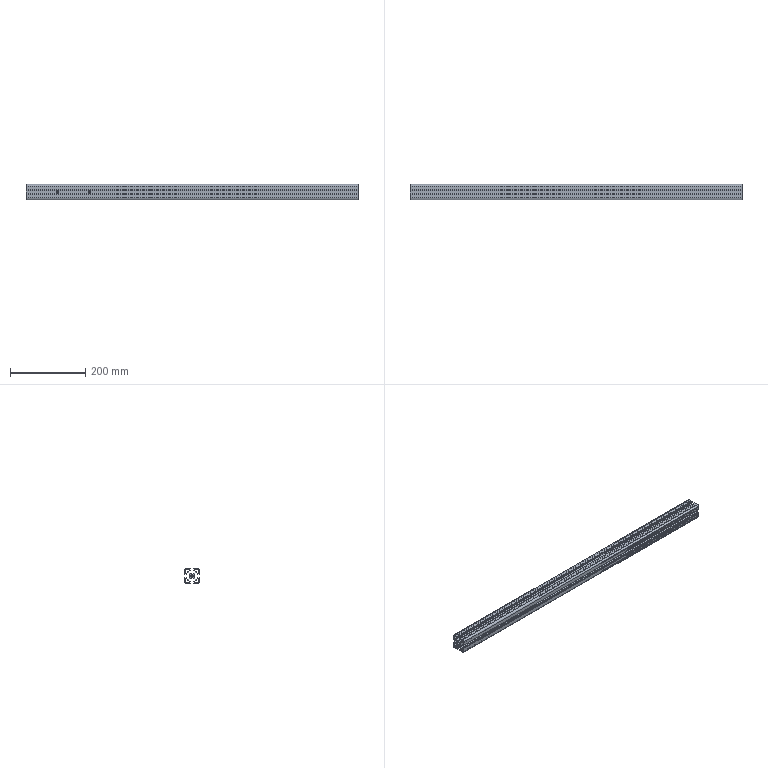Part | STEP file | 1 solid | 226 faces | box 880 x 40 x 40 mm | volume 420476 mm3 | cylinder 120 | plane 106 | commonest cylinder face diameters 0.6 x38 2 x28 4 x16 10 x10 0.4 x8 5.8 x8